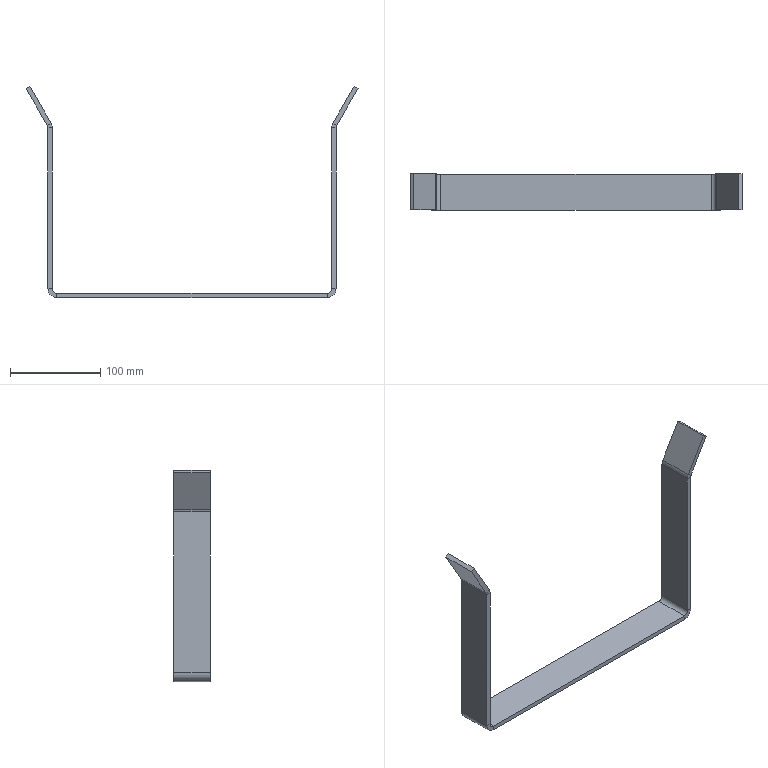Part | SolidWorks | features EdgeFlange 2, FlatPattern 1, SMBaseFlange 1, SheetMetal 1 | 1 solid | 38 faces | box 368.66 x 40 x 234.641 mm | volume 156675 mm3 | plane 30 | cylinder 8 | commonest cylinder face diameters 10 x4 20 x4
STEP:
#1=CARTESIAN_POINT('',(160.,-20.,5.));
#2=VERTEX_POINT('',#1);
#3=CARTESIAN_POINT('',(160.,-20.,183.66));
#4=VERTEX_POINT('',#3);
#5=CARTESIAN_POINT('',(160.,-20.,0.));
#6=DIRECTION('',(0.,0.,1.));
#7=VECTOR('',#6,1000.);
#8=LINE('',#5,#7);
#9=EDGE_CURVE('',#2,#4,#8,.T.);
#10=ORIENTED_EDGE('',*,*,#9,.T.);
#11=CARTESIAN_POINT('',(155.,-20.,183.66));
#12=VERTEX_POINT('',#11);
#13=CARTESIAN_POINT('',(160.,-20.,183.66));
#14=DIRECTION('',(-1.,0.,0.));
#15=VECTOR('',#14,1000.);
#16=LINE('',#13,#15);
#17=EDGE_CURVE('',#4,#12,#16,.T.);
#18=ORIENTED_EDGE('',*,*,#17,.T.);
#19=CARTESIAN_POINT('',(155.,-20.,5.));
#20=VERTEX_POINT('',#19);
#21=CARTESIAN_POINT('',(155.,-20.,0.));
#22=DIRECTION('',(0.,0.,1.));
#23=VECTOR('',#22,1000.);
#24=LINE('',#21,#23);
#25=EDGE_CURVE('',#20,#12,#24,.T.);
#26=ORIENTED_EDGE('',*,*,#25,.F.);
#27=CARTESIAN_POINT('',(160.,-20.,5.));
#28=DIRECTION('',(1.,0.,0.));
#29=VECTOR('',#28,1000.);
#30=LINE('',#27,#29);
#31=EDGE_CURVE('',#20,#2,#30,.T.);
#32=ORIENTED_EDGE('',*,*,#31,.T.);
#33=EDGE_LOOP('',(#10,#18,#26,#32));
#34=FACE_OUTER_BOUND('',#33,.T.);
#35=CARTESIAN_POINT('',(160.,-20.,0.));
#36=DIRECTION('',(0.,-1.,0.));
#37=DIRECTION('',(0.,0.,-1.));
#38=AXIS2_PLACEMENT_3D('',#35,#36,#37);
#39=PLANE('',#38);
#40=ADVANCED_FACE('',(#34),#39,.T.);
#41=CARTESIAN_POINT('',(160.,20.,183.66));
#42=VERTEX_POINT('',#41);
#43=CARTESIAN_POINT('',(160.,-20.,183.66));
#44=DIRECTION('',(0.,1.,0.));
#45=VECTOR('',#44,1000.);
#46=LINE('',#43,#45);
#47=EDGE_CURVE('',#4,#42,#46,.T.);
#48=ORIENTED_EDGE('',*,*,#47,.F.);
#49=ORIENTED_EDGE('',*,*,#9,.F.);
#50=CARTESIAN_POINT('',(160.,20.,5.));
#51=VERTEX_POINT('',#50);
#52=CARTESIAN_POINT('',(160.,-20.,5.));
#53=DIRECTION('',(0.,-1.,0.));
#54=VECTOR('',#53,1000.);
#55=LINE('',#52,#54);
#56=EDGE_CURVE('',#51,#2,#55,.T.);
#57=ORIENTED_EDGE('',*,*,#56,.F.);
#58=CARTESIAN_POINT('',(160.,20.,195.));
#59=DIRECTION('',(0.,0.,-1.));
#60=VECTOR('',#59,1000.);
#61=LINE('',#58,#60);
#62=EDGE_CURVE('',#42,#51,#61,.T.);
#63=ORIENTED_EDGE('',*,*,#62,.F.);
#64=EDGE_LOOP('',(#48,#49,#57,#63));
#65=FACE_OUTER_BOUND('',#64,.T.);
#66=CARTESIAN_POINT('',(160.,0.,0.));
#67=DIRECTION('',(-1.,0.,0.));
#68=DIRECTION('',(0.,0.,1.));
#69=AXIS2_PLACEMENT_3D('',#66,#67,#68);
#70=PLANE('',#69);
#71=ADVANCED_FACE('',(#65),#70,.F.);
#72=ORIENTED_EDGE('',*,*,#25,.T.);
#73=CARTESIAN_POINT('',(155.,20.,183.66));
#74=VERTEX_POINT('',#73);
#75=CARTESIAN_POINT('',(155.,-20.,183.66));
#76=DIRECTION('',(0.,1.,0.));
#77=VECTOR('',#76,1000.);
#78=LINE('',#75,#77);
#79=EDGE_CURVE('',#12,#74,#78,.T.);
#80=ORIENTED_EDGE('',*,*,#79,.T.);
#81=CARTESIAN_POINT('',(155.,20.,5.));
#82=VERTEX_POINT('',#81);
#83=CARTESIAN_POINT('',(155.,20.,0.));
#84=DIRECTION('',(0.,0.,-1.));
#85=VECTOR('',#84,1000.);
#86=LINE('',#83,#85);
#87=EDGE_CURVE('',#74,#82,#86,.T.);
#88=ORIENTED_EDGE('',*,*,#87,.T.);
#89=CARTESIAN_POINT('',(155.,-20.,5.));
#90=DIRECTION('',(0.,1.,0.));
#91=VECTOR('',#90,1000.);
#92=LINE('',#89,#91);
#93=EDGE_CURVE('',#20,#82,#92,.T.);
#94=ORIENTED_EDGE('',*,*,#93,.F.);
#95=EDGE_LOOP('',(#72,#80,#88,#94));
#96=FACE_OUTER_BOUND('',#95,.T.);
#97=CARTESIAN_POINT('',(155.,0.,0.));
#98=DIRECTION('',(-1.,0.,0.));
#99=DIRECTION('',(0.,0.,1.));
#100=AXIS2_PLACEMENT_3D('',#97,#98,#99);
#101=PLANE('',#100);
#102=ADVANCED_FACE('',(#96),#101,.T.);
#103=CARTESIAN_POINT('',(-160.,20.,5.));
#104=VERTEX_POINT('',#103);
#105=CARTESIAN_POINT('',(-160.,20.,183.66));
#106=VERTEX_POINT('',#105);
#107=CARTESIAN_POINT('',(-160.,20.,195.));
#108=DIRECTION('',(0.,0.,1.));
#109=VECTOR('',#108,1000.);
#110=LINE('',#107,#109);
#111=EDGE_CURVE('',#104,#106,#110,.T.);
#112=ORIENTED_EDGE('',*,*,#111,.T.);
#113=CARTESIAN_POINT('',(-155.,20.,183.66));
#114=VERTEX_POINT('',#113);
#115=CARTESIAN_POINT('',(-160.,20.,183.66));
#116=DIRECTION('',(1.,0.,0.));
#117=VECTOR('',#116,1000.);
#118=LINE('',#115,#117);
#119=EDGE_CURVE('',#106,#114,#118,.T.);
#120=ORIENTED_EDGE('',*,*,#119,.T.);
#121=CARTESIAN_POINT('',(-155.,20.,5.));
#122=VERTEX_POINT('',#121);
#123=CARTESIAN_POINT('',(-155.,20.,0.));
#124=DIRECTION('',(0.,0.,1.));
#125=VECTOR('',#124,1000.);
#126=LINE('',#123,#125);
#127=EDGE_CURVE('',#122,#114,#126,.T.);
#128=ORIENTED_EDGE('',*,*,#127,.F.);
#129=CARTESIAN_POINT('',(-160.,20.,5.));
#130=DIRECTION('',(-1.,0.,0.));
#131=VECTOR('',#130,1000.);
#132=LINE('',#129,#131);
#133=EDGE_CURVE('',#122,#104,#132,.T.);
#134=ORIENTED_EDGE('',*,*,#133,.T.);
#135=EDGE_LOOP('',(#112,#120,#128,#134));
#136=FACE_OUTER_BOUND('',#135,.T.);
#137=CARTESIAN_POINT('',(-160.,20.,195.));
#138=DIRECTION('',(0.,1.,0.));
#139=DIRECTION('',(0.,0.,1.));
#140=AXIS2_PLACEMENT_3D('',#137,#138,#139);
#141=PLANE('',#140);
#142=ADVANCED_FACE('',(#136),#141,.T.);
#143=CARTESIAN_POINT('',(-160.,-20.,183.66));
#144=VERTEX_POINT('',#143);
#145=CARTESIAN_POINT('',(-160.,-20.,5.));
#146=VERTEX_POINT('',#145);
#147=CARTESIAN_POINT('',(-160.,-20.,0.));
#148=DIRECTION('',(0.,0.,-1.));
#149=VECTOR('',#148,1000.);
#150=LINE('',#147,#149);
#151=EDGE_CURVE('',#144,#146,#150,.T.);
#152=ORIENTED_EDGE('',*,*,#151,.F.);
#153=CARTESIAN_POINT('',(-160.,20.,183.66));
#154=DIRECTION('',(0.,-1.,0.));
#155=VECTOR('',#154,1000.);
#156=LINE('',#153,#155);
#157=EDGE_CURVE('',#106,#144,#156,.T.);
#158=ORIENTED_EDGE('',*,*,#157,.F.);
#159=ORIENTED_EDGE('',*,*,#111,.F.);
#160=CARTESIAN_POINT('',(-160.,0.,5.));
#161=DIRECTION('',(0.,-1.,0.));
#162=VECTOR('',#161,1000.);
#163=LINE('',#160,#162);
#164=EDGE_CURVE('',#104,#146,#163,.T.);
#165=ORIENTED_EDGE('',*,*,#164,.T.);
#166=EDGE_LOOP('',(#152,#158,#159,#165));
#167=FACE_OUTER_BOUND('',#166,.T.);
#168=CARTESIAN_POINT('',(-160.,0.,0.));
#169=DIRECTION('',(-1.,0.,0.));
#170=DIRECTION('',(0.,0.,1.));
#171=AXIS2_PLACEMENT_3D('',#168,#169,#170);
#172=PLANE('',#171);
#173=ADVANCED_FACE('',(#167),#172,.T.);
#174=CARTESIAN_POINT('',(-155.,-20.,183.66));
#175=VERTEX_POINT('',#174);
#176=CARTESIAN_POINT('',(-155.,20.,183.66));
#177=DIRECTION('',(0.,-1.,0.));
#178=VECTOR('',#177,1000.);
#179=LINE('',#176,#178);
#180=EDGE_CURVE('',#114,#175,#179,.T.);
#181=ORIENTED_EDGE('',*,*,#180,.T.);
#182=CARTESIAN_POINT('',(-155.,-20.,5.));
#183=VERTEX_POINT('',#182);
#184=CARTESIAN_POINT('',(-155.,-20.,0.));
#185=DIRECTION('',(0.,0.,-1.));
#186=VECTOR('',#185,1000.);
#187=LINE('',#184,#186);
#188=EDGE_CURVE('',#175,#183,#187,.T.);
#189=ORIENTED_EDGE('',*,*,#188,.T.);
#190=CARTESIAN_POINT('',(-155.,20.,5.));
#191=DIRECTION('',(0.,-1.,0.));
#192=VECTOR('',#191,1000.);
#193=LINE('',#190,#192);
#194=EDGE_CURVE('',#122,#183,#193,.T.);
#195=ORIENTED_EDGE('',*,*,#194,.F.);
#196=ORIENTED_EDGE('',*,*,#127,.T.);
#197=EDGE_LOOP('',(#181,#189,#195,#196));
#198=FACE_OUTER_BOUND('',#197,.T.);
#199=CARTESIAN_POINT('',(-155.,0.,0.));
#200=DIRECTION('',(-1.,0.,0.));
#201=DIRECTION('',(0.,0.,1.));
#202=AXIS2_PLACEMENT_3D('',#199,#200,#201);
#203=PLANE('',#202);
#204=ADVANCED_FACE('',(#198),#203,.F.);
#205=CARTESIAN_POINT('',(150.,20.,-5.));
#206=VERTEX_POINT('',#205);
#207=CARTESIAN_POINT('',(150.,-20.,-5.));
#208=VERTEX_POINT('',#207);
#209=CARTESIAN_POINT('',(150.,20.,-5.));
#210=DIRECTION('',(0.,-1.,0.));
#211=VECTOR('',#210,1000.);
#212=LINE('',#209,#211);
#213=EDGE_CURVE('',#206,#208,#212,.T.);
#214=ORIENTED_EDGE('',*,*,#213,.T.);
#215=CARTESIAN_POINT('',(-150.,-20.,-5.));
#216=VERTEX_POINT('',#215);
#217=CARTESIAN_POINT('',(-160.,-20.,-5.));
#218=DIRECTION('',(1.,0.,0.));
#219=VECTOR('',#218,1000.);
#220=LINE('',#217,#219);
#221=EDGE_CURVE('',#216,#208,#220,.T.);
#222=ORIENTED_EDGE('',*,*,#221,.F.);
#223=CARTESIAN_POINT('',(-150.,20.,-5.));
#224=VERTEX_POINT('',#223);
#225=CARTESIAN_POINT('',(-150.,-20.,-5.));
#226=DIRECTION('',(0.,1.,0.));
#227=VECTOR('',#226,1000.);
#228=LINE('',#225,#227);
#229=EDGE_CURVE('',#216,#224,#228,.T.);
#230=ORIENTED_EDGE('',*,*,#229,.T.);
#231=CARTESIAN_POINT('',(-160.,20.,-5.));
#232=DIRECTION('',(-1.,0.,0.));
#233=VECTOR('',#232,1000.);
#234=LINE('',#231,#233);
#235=EDGE_CURVE('',#206,#224,#234,.T.);
#236=ORIENTED_EDGE('',*,*,#235,.F.);
#237=EDGE_LOOP('',(#214,#222,#230,#236));
#238=FACE_OUTER_BOUND('',#237,.T.);
#239=CARTESIAN_POINT('',(0.,0.,-5.));
#240=DIRECTION('',(0.,0.,1.));
#241=DIRECTION('',(1.,0.,0.));
#242=AXIS2_PLACEMENT_3D('',#239,#240,#241);
#243=PLANE('',#242);
#244=ADVANCED_FACE('',(#238),#243,.F.);
#245=CARTESIAN_POINT('',(-150.,-20.,0.));
#246=VERTEX_POINT('',#245);
#247=CARTESIAN_POINT('',(150.,-20.,0.));
#248=VERTEX_POINT('',#247);
#249=CARTESIAN_POINT('',(-160.,-20.,0.));
#250=DIRECTION('',(1.,0.,0.));
#251=VECTOR('',#250,1000.);
#252=LINE('',#249,#251);
#253=EDGE_CURVE('',#246,#248,#252,.T.);
#254=ORIENTED_EDGE('',*,*,#253,.T.);
#255=CARTESIAN_POINT('',(150.,20.,0.));
#256=VERTEX_POINT('',#255);
#257=CARTESIAN_POINT('',(150.,20.,0.));
#258=DIRECTION('',(0.,-1.,0.));
#259=VECTOR('',#258,1000.);
#260=LINE('',#257,#259);
#261=EDGE_CURVE('',#256,#248,#260,.T.);
#262=ORIENTED_EDGE('',*,*,#261,.F.);
#263=CARTESIAN_POINT('',(-150.,20.,0.));
#264=VERTEX_POINT('',#263);
#265=CARTESIAN_POINT('',(-160.,20.,0.));
#266=DIRECTION('',(-1.,0.,0.));
#267=VECTOR('',#266,1000.);
#268=LINE('',#265,#267);
#269=EDGE_CURVE('',#256,#264,#268,.T.);
#270=ORIENTED_EDGE('',*,*,#269,.T.);
#271=CARTESIAN_POINT('',(-150.,-20.,0.));
#272=DIRECTION('',(0.,1.,0.));
#273=VECTOR('',#272,1000.);
#274=LINE('',#271,#273);
#275=EDGE_CURVE('',#246,#264,#274,.T.);
#276=ORIENTED_EDGE('',*,*,#275,.F.);
#277=EDGE_LOOP('',(#254,#262,#270,#276));
#278=FACE_OUTER_BOUND('',#277,.T.);
#279=CARTESIAN_POINT('',(0.,0.,0.));
#280=DIRECTION('',(0.,0.,1.));
#281=DIRECTION('',(1.,0.,0.));
#282=AXIS2_PLACEMENT_3D('',#279,#280,#281);
#283=PLANE('',#282);
#284=ADVANCED_FACE('',(#278),#283,.T.);
#285=ORIENTED_EDGE('',*,*,#269,.F.);
#286=CARTESIAN_POINT('',(150.,20.,0.));
#287=DIRECTION('',(0.,0.,-1.));
#288=VECTOR('',#287,1000.);
#289=LINE('',#286,#288);
#290=EDGE_CURVE('',#256,#206,#289,.T.);
#291=ORIENTED_EDGE('',*,*,#290,.T.);
#292=ORIENTED_EDGE('',*,*,#235,.T.);
#293=CARTESIAN_POINT('',(-150.,20.,0.));
#294=DIRECTION('',(0.,0.,-1.));
#295=VECTOR('',#294,1000.);
#296=LINE('',#293,#295);
#297=EDGE_CURVE('',#264,#224,#296,.T.);
#298=ORIENTED_EDGE('',*,*,#297,.F.);
#299=EDGE_LOOP('',(#285,#291,#292,#298));
#300=FACE_OUTER_BOUND('',#299,.T.);
#301=CARTESIAN_POINT('',(-160.,20.,-5.));
#302=DIRECTION('',(0.,1.,0.));
#303=DIRECTION('',(0.,0.,1.));
#304=AXIS2_PLACEMENT_3D('',#301,#302,#303);
#305=PLANE('',#304);
#306=ADVANCED_FACE('',(#300),#305,.T.);
#307=CARTESIAN_POINT('',(150.,-20.,0.));
#308=DIRECTION('',(0.,0.,-1.));
#309=VECTOR('',#308,1000.);
#310=LINE('',#307,#309);
#311=EDGE_CURVE('',#248,#208,#310,.T.);
#312=ORIENTED_EDGE('',*,*,#311,.F.);
#313=ORIENTED_EDGE('',*,*,#253,.F.);
#314=CARTESIAN_POINT('',(-150.,-20.,0.));
#315=DIRECTION('',(0.,0.,-1.));
#316=VECTOR('',#315,1000.);
#317=LINE('',#314,#316);
#318=EDGE_CURVE('',#246,#216,#317,.T.);
#319=ORIENTED_EDGE('',*,*,#318,.T.);
#320=ORIENTED_EDGE('',*,*,#221,.T.);
#321=EDGE_LOOP('',(#312,#313,#319,#320));
#322=FACE_OUTER_BOUND('',#321,.T.);
#323=CARTESIAN_POINT('',(-160.,-20.,-5.));
#324=DIRECTION('',(0.,-1.,0.));
#325=DIRECTION('',(0.,0.,-1.));
#326=AXIS2_PLACEMENT_3D('',#323,#324,#325);
#327=PLANE('',#326);
#328=ADVANCED_FACE('',(#322),#327,.T.);
#329=ORIENTED_EDGE('',*,*,#133,.F.);
#330=CARTESIAN_POINT('',(-150.,20.,5.));
#331=DIRECTION('',(0.,1.,0.));
#332=DIRECTION('',(0.,0.,-1.));
#333=AXIS2_PLACEMENT_3D('',#330,#331,#332);
#334=CIRCLE('',#333,5.);
#335=EDGE_CURVE('',#264,#122,#334,.T.);
#336=ORIENTED_EDGE('',*,*,#335,.F.);
#337=ORIENTED_EDGE('',*,*,#297,.T.);
#338=CARTESIAN_POINT('',(-150.,20.,5.));
#339=DIRECTION('',(0.,1.,0.));
#340=DIRECTION('',(0.,0.,-1.));
#341=AXIS2_PLACEMENT_3D('',#338,#339,#340);
#342=CIRCLE('',#341,10.);
#343=EDGE_CURVE('',#224,#104,#342,.T.);
#344=ORIENTED_EDGE('',*,*,#343,.T.);
#345=EDGE_LOOP('',(#329,#336,#337,#344));
#346=FACE_OUTER_BOUND('',#345,.T.);
#347=CARTESIAN_POINT('',(-150.,20.,5.));
#348=DIRECTION('',(0.,1.,0.));
#349=DIRECTION('',(0.,0.,1.));
#350=AXIS2_PLACEMENT_3D('',#347,#348,#349);
#351=PLANE('',#350);
#352=ADVANCED_FACE('',(#346),#351,.T.);
#353=CARTESIAN_POINT('',(-150.,-20.,5.));
#354=DIRECTION('',(0.,-1.,0.));
#355=DIRECTION('',(0.,0.,-1.));
#356=AXIS2_PLACEMENT_3D('',#353,#354,#355);
#357=CIRCLE('',#356,5.);
#358=EDGE_CURVE('',#183,#246,#357,.T.);
#359=ORIENTED_EDGE('',*,*,#358,.F.);
#360=CARTESIAN_POINT('',(-155.,-20.,5.));
#361=DIRECTION('',(-1.,0.,0.));
#362=VECTOR('',#361,1000.);
#363=LINE('',#360,#362);
#364=EDGE_CURVE('',#183,#146,#363,.T.);
#365=ORIENTED_EDGE('',*,*,#364,.T.);
#366=CARTESIAN_POINT('',(-150.,-20.,5.));
#367=DIRECTION('',(0.,-1.,0.));
#368=DIRECTION('',(0.,0.,-1.));
#369=AXIS2_PLACEMENT_3D('',#366,#367,#368);
#370=CIRCLE('',#369,10.);
#371=EDGE_CURVE('',#146,#216,#370,.T.);
#372=ORIENTED_EDGE('',*,*,#371,.T.);
#373=ORIENTED_EDGE('',*,*,#318,.F.);
#374=EDGE_LOOP('',(#359,#365,#372,#373));
#375=FACE_OUTER_BOUND('',#374,.T.);
#376=CARTESIAN_POINT('',(-150.,-20.,5.));
#377=DIRECTION('',(0.,1.,0.));
#378=DIRECTION('',(0.,0.,1.));
#379=AXIS2_PLACEMENT_3D('',#376,#377,#378);
#380=PLANE('',#379);
#381=ADVANCED_FACE('',(#375),#380,.F.);
#382=ORIENTED_EDGE('',*,*,#229,.F.);
#383=ORIENTED_EDGE('',*,*,#371,.F.);
#384=ORIENTED_EDGE('',*,*,#164,.F.);
#385=ORIENTED_EDGE('',*,*,#343,.F.);
#386=EDGE_LOOP('',(#382,#383,#384,#385));
#387=FACE_OUTER_BOUND('',#386,.T.);
#388=CARTESIAN_POINT('',(-150.,-20.,5.));
#389=DIRECTION('',(0.,-1.,0.));
#390=DIRECTION('',(-1.,0.,0.));
#391=AXIS2_PLACEMENT_3D('',#388,#389,#390);
#392=CYLINDRICAL_SURFACE('',#391,10.);
#393=ADVANCED_FACE('',(#387),#392,.T.);
#394=ORIENTED_EDGE('',*,*,#275,.T.);
#395=ORIENTED_EDGE('',*,*,#335,.T.);
#396=ORIENTED_EDGE('',*,*,#194,.T.);
#397=ORIENTED_EDGE('',*,*,#358,.T.);
#398=EDGE_LOOP('',(#394,#395,#396,#397));
#399=FACE_OUTER_BOUND('',#398,.T.);
#400=CARTESIAN_POINT('',(-150.,-20.,5.));
#401=DIRECTION('',(0.,-1.,0.));
#402=DIRECTION('',(-1.,0.,0.));
#403=AXIS2_PLACEMENT_3D('',#400,#401,#402);
#404=CYLINDRICAL_SURFACE('',#403,5.);
#405=ADVANCED_FACE('',(#399),#404,.F.);
#406=CARTESIAN_POINT('',(-160.,-20.,183.66));
#407=DIRECTION('',(1.,0.,0.));
#408=VECTOR('',#407,1000.);
#409=LINE('',#406,#408);
#410=EDGE_CURVE('',#144,#175,#409,.T.);
#411=ORIENTED_EDGE('',*,*,#410,.F.);
#412=ORIENTED_EDGE('',*,*,#151,.T.);
#413=ORIENTED_EDGE('',*,*,#364,.F.);
#414=ORIENTED_EDGE('',*,*,#188,.F.);
#415=EDGE_LOOP('',(#411,#412,#413,#414));
#416=FACE_OUTER_BOUND('',#415,.T.);
#417=CARTESIAN_POINT('',(-160.,-20.,0.));
#418=DIRECTION('',(0.,-1.,0.));
#419=DIRECTION('',(0.,0.,-1.));
#420=AXIS2_PLACEMENT_3D('',#417,#418,#419);
#421=PLANE('',#420);
#422=ADVANCED_FACE('',(#416),#421,.T.);
#423=ORIENTED_EDGE('',*,*,#31,.F.);
#424=CARTESIAN_POINT('',(150.,-20.,5.));
#425=DIRECTION('',(0.,-1.,0.));
#426=DIRECTION('',(0.,0.,1.));
#427=AXIS2_PLACEMENT_3D('',#424,#425,#426);
#428=CIRCLE('',#427,5.);
#429=EDGE_CURVE('',#248,#20,#428,.T.);
#430=ORIENTED_EDGE('',*,*,#429,.F.);
#431=ORIENTED_EDGE('',*,*,#311,.T.);
#432=CARTESIAN_POINT('',(150.,-20.,5.));
#433=DIRECTION('',(0.,-1.,0.));
#434=DIRECTION('',(0.,0.,1.));
#435=AXIS2_PLACEMENT_3D('',#432,#433,#434);
#436=CIRCLE('',#435,10.);
#437=EDGE_CURVE('',#208,#2,#436,.T.);
#438=ORIENTED_EDGE('',*,*,#437,.T.);
#439=EDGE_LOOP('',(#423,#430,#431,#438));
#440=FACE_OUTER_BOUND('',#439,.T.);
#441=CARTESIAN_POINT('',(150.,-20.,5.));
#442=DIRECTION('',(0.,-1.,0.));
#443=DIRECTION('',(0.,0.,-1.));
#444=AXIS2_PLACEMENT_3D('',#441,#442,#443);
#445=PLANE('',#444);
#446=ADVANCED_FACE('',(#440),#445,.T.);
#447=CARTESIAN_POINT('',(150.,20.,5.));
#448=DIRECTION('',(0.,1.,0.));
#449=DIRECTION('',(0.,0.,1.));
#450=AXIS2_PLACEMENT_3D('',#447,#448,#449);
#451=CIRCLE('',#450,5.);
#452=EDGE_CURVE('',#82,#256,#451,.T.);
#453=ORIENTED_EDGE('',*,*,#452,.F.);
#454=CARTESIAN_POINT('',(155.,20.,5.));
#455=DIRECTION('',(1.,0.,0.));
#456=VECTOR('',#455,1000.);
#457=LINE('',#454,#456);
#458=EDGE_CURVE('',#82,#51,#457,.T.);
#459=ORIENTED_EDGE('',*,*,#458,.T.);
#460=CARTESIAN_POINT('',(150.,20.,5.));
#461=DIRECTION('',(0.,1.,0.));
#462=DIRECTION('',(0.,0.,1.));
#463=AXIS2_PLACEMENT_3D('',#460,#461,#462);
#464=CIRCLE('',#463,10.);
#465=EDGE_CURVE('',#51,#206,#464,.T.);
#466=ORIENTED_EDGE('',*,*,#465,.T.);
#467=ORIENTED_EDGE('',*,*,#290,.F.);
#468=EDGE_LOOP('',(#453,#459,#466,#467));
#469=FACE_OUTER_BOUND('',#468,.T.);
#470=CARTESIAN_POINT('',(150.,20.,5.));
#471=DIRECTION('',(0.,-1.,0.));
#472=DIRECTION('',(0.,0.,-1.));
#473=AXIS2_PLACEMENT_3D('',#470,#471,#472);
#474=PLANE('',#473);
#475=ADVANCED_FACE('',(#469),#474,.F.);
#476=ORIENTED_EDGE('',*,*,#213,.F.);
#477=ORIENTED_EDGE('',*,*,#465,.F.);
#478=ORIENTED_EDGE('',*,*,#56,.T.);
#479=ORIENTED_EDGE('',*,*,#437,.F.);
#480=EDGE_LOOP('',(#476,#477,#478,#479));
#481=FACE_OUTER_BOUND('',#480,.T.);
#482=CARTESIAN_POINT('',(150.,20.,5.));
#483=DIRECTION('',(0.,1.,0.));
#484=DIRECTION('',(1.,0.,0.));
#485=AXIS2_PLACEMENT_3D('',#482,#483,#484);
#486=CYLINDRICAL_SURFACE('',#485,10.);
#487=ADVANCED_FACE('',(#481),#486,.T.);
#488=ORIENTED_EDGE('',*,*,#261,.T.);
#489=ORIENTED_EDGE('',*,*,#429,.T.);
#490=ORIENTED_EDGE('',*,*,#93,.T.);
#491=ORIENTED_EDGE('',*,*,#452,.T.);
#492=EDGE_LOOP('',(#488,#489,#490,#491));
#493=FACE_OUTER_BOUND('',#492,.T.);
#494=CARTESIAN_POINT('',(150.,20.,5.));
#495=DIRECTION('',(0.,1.,0.));
#496=DIRECTION('',(1.,0.,0.));
#497=AXIS2_PLACEMENT_3D('',#494,#495,#496);
#498=CYLINDRICAL_SURFACE('',#497,5.);
#499=ADVANCED_FACE('',(#493),#498,.F.);
#500=CARTESIAN_POINT('',(160.,20.,183.66));
#501=DIRECTION('',(-1.,0.,0.));
#502=VECTOR('',#501,1000.);
#503=LINE('',#500,#502);
#504=EDGE_CURVE('',#42,#74,#503,.T.);
#505=ORIENTED_EDGE('',*,*,#504,.F.);
#506=ORIENTED_EDGE('',*,*,#62,.T.);
#507=ORIENTED_EDGE('',*,*,#458,.F.);
#508=ORIENTED_EDGE('',*,*,#87,.F.);
#509=EDGE_LOOP('',(#505,#506,#507,#508));
#510=FACE_OUTER_BOUND('',#509,.T.);
#511=CARTESIAN_POINT('',(160.,20.,195.));
#512=DIRECTION('',(0.,1.,0.));
#513=DIRECTION('',(0.,0.,1.));
#514=AXIS2_PLACEMENT_3D('',#511,#512,#513);
#515=PLANE('',#514);
#516=ADVANCED_FACE('',(#510),#515,.T.);
#517=CARTESIAN_POINT('',(-160.67,-20.,186.16));
#518=VERTEX_POINT('',#517);
#519=CARTESIAN_POINT('',(-156.34,-20.,188.66));
#520=VERTEX_POINT('',#519);
#521=CARTESIAN_POINT('',(-156.34,-20.,188.66));
#522=DIRECTION('',(0.866,0.,0.5));
#523=VECTOR('',#522,1000.);
#524=LINE('',#521,#523);
#525=EDGE_CURVE('',#518,#520,#524,.T.);
#526=ORIENTED_EDGE('',*,*,#525,.F.);
#527=CARTESIAN_POINT('',(-165.,-20.,183.66));
#528=DIRECTION('',(0.,-1.,0.));
#529=DIRECTION('',(0.,0.,1.));
#530=AXIS2_PLACEMENT_3D('',#527,#528,#529);
#531=CIRCLE('',#530,5.);
#532=EDGE_CURVE('',#144,#518,#531,.T.);
#533=ORIENTED_EDGE('',*,*,#532,.F.);
#534=ORIENTED_EDGE('',*,*,#410,.T.);
#535=CARTESIAN_POINT('',(-165.,-20.,183.66));
#536=DIRECTION('',(0.,-1.,0.));
#537=DIRECTION('',(0.,0.,1.));
#538=AXIS2_PLACEMENT_3D('',#535,#536,#537);
#539=CIRCLE('',#538,10.);
#540=EDGE_CURVE('',#175,#520,#539,.T.);
#541=ORIENTED_EDGE('',*,*,#540,.T.);
#542=EDGE_LOOP('',(#526,#533,#534,#541));
#543=FACE_OUTER_BOUND('',#542,.T.);
#544=CARTESIAN_POINT('',(-165.,-20.,183.66));
#545=DIRECTION('',(0.,-1.,0.));
#546=DIRECTION('',(0.,0.,-1.));
#547=AXIS2_PLACEMENT_3D('',#544,#545,#546);
#548=PLANE('',#547);
#549=ADVANCED_FACE('',(#543),#548,.T.);
#550=CARTESIAN_POINT('',(-160.67,20.,186.16));
#551=VERTEX_POINT('',#550);
#552=CARTESIAN_POINT('',(-165.,20.,183.66));
#553=DIRECTION('',(0.,1.,0.));
#554=DIRECTION('',(0.,0.,1.));
#555=AXIS2_PLACEMENT_3D('',#552,#553,#554);
#556=CIRCLE('',#555,5.);
#557=EDGE_CURVE('',#551,#106,#556,.T.);
#558=ORIENTED_EDGE('',*,*,#557,.F.);
#559=CARTESIAN_POINT('',(-156.34,20.,188.66));
#560=VERTEX_POINT('',#559);
#561=CARTESIAN_POINT('',(-160.67,20.,186.16));
#562=DIRECTION('',(0.866,0.,0.5));
#563=VECTOR('',#562,1000.);
#564=LINE('',#561,#563);
#565=EDGE_CURVE('',#551,#560,#564,.T.);
#566=ORIENTED_EDGE('',*,*,#565,.T.);
#567=CARTESIAN_POINT('',(-165.,20.,183.66));
#568=DIRECTION('',(0.,1.,0.));
#569=DIRECTION('',(0.,0.,1.));
#570=AXIS2_PLACEMENT_3D('',#567,#568,#569);
#571=CIRCLE('',#570,10.);
#572=EDGE_CURVE('',#560,#114,#571,.T.);
#573=ORIENTED_EDGE('',*,*,#572,.T.);
#574=ORIENTED_EDGE('',*,*,#119,.F.);
#575=EDGE_LOOP('',(#558,#566,#573,#574));
#576=FACE_OUTER_BOUND('',#575,.T.);
#577=CARTESIAN_POINT('',(-165.,20.,183.66));
#578=DIRECTION('',(0.,-1.,0.));
#579=DIRECTION('',(0.,0.,-1.));
#580=AXIS2_PLACEMENT_3D('',#577,#578,#579);
#581=PLANE('',#580);
#582=ADVANCED_FACE('',(#576),#581,.F.);
#583=ORIENTED_EDGE('',*,*,#180,.F.);
#584=ORIENTED_EDGE('',*,*,#572,.F.);
#585=CARTESIAN_POINT('',(-156.34,0.,188.66));
#586=DIRECTION('',(0.,1.,0.));
#587=VECTOR('',#586,1000.);
#588=LINE('',#585,#587);
#589=EDGE_CURVE('',#520,#560,#588,.T.);
#590=ORIENTED_EDGE('',*,*,#589,.F.);
#591=ORIENTED_EDGE('',*,*,#540,.F.);
#592=EDGE_LOOP('',(#583,#584,#590,#591));
#593=FACE_OUTER_BOUND('',#592,.T.);
#594=CARTESIAN_POINT('',(-165.,20.,183.66));
#595=DIRECTION('',(0.,1.,0.));
#596=DIRECTION('',(0.866,0.,0.5));
#597=AXIS2_PLACEMENT_3D('',#594,#595,#596);
#598=CYLINDRICAL_SURFACE('',#597,10.);
#599=ADVANCED_FACE('',(#593),#598,.T.);
#600=ORIENTED_EDGE('',*,*,#157,.T.);
#601=ORIENTED_EDGE('',*,*,#532,.T.);
#602=CARTESIAN_POINT('',(-160.67,-20.,186.16));
#603=DIRECTION('',(0.,1.,0.));
#604=VECTOR('',#603,1000.);
#605=LINE('',#602,#604);
#606=EDGE_CURVE('',#518,#551,#605,.T.);
#607=ORIENTED_EDGE('',*,*,#606,.T.);
#608=ORIENTED_EDGE('',*,*,#557,.T.);
#609=EDGE_LOOP('',(#600,#601,#607,#608));
#610=FACE_OUTER_BOUND('',#609,.T.);
#611=CARTESIAN_POINT('',(-165.,20.,183.66));
#612=DIRECTION('',(0.,1.,0.));
#613=DIRECTION('',(0.866,0.,0.5));
#614=AXIS2_PLACEMENT_3D('',#611,#612,#613);
#615=CYLINDRICAL_SURFACE('',#614,5.);
#616=ADVANCED_FACE('',(#610),#615,.F.);
#617=CARTESIAN_POINT('',(-180.,20.,229.641));
#618=VERTEX_POINT('',#617);
#619=CARTESIAN_POINT('',(-155.67,20.,187.5));
#620=DIRECTION('',(0.5,0.,-0.866));
#621=VECTOR('',#620,1000.);
#622=LINE('',#619,#621);
#623=EDGE_CURVE('',#618,#560,#622,.T.);
#624=ORIENTED_EDGE('',*,*,#623,.T.);
#625=ORIENTED_EDGE('',*,*,#565,.F.);
#626=CARTESIAN_POINT('',(-184.33,20.,227.141));
#627=VERTEX_POINT('',#626);
#628=CARTESIAN_POINT('',(-35.563,20.,-30.532));
#629=DIRECTION('',(0.5,0.,-0.866));
#630=VECTOR('',#629,1000.);
#631=LINE('',#628,#630);
#632=EDGE_CURVE('',#627,#551,#631,.T.);
#633=ORIENTED_EDGE('',*,*,#632,.F.);
#634=CARTESIAN_POINT('',(-180.,20.,229.641));
#635=DIRECTION('',(-0.866,0.,-0.5));
#636=VECTOR('',#635,1000.);
#637=LINE('',#634,#636);
#638=EDGE_CURVE('',#618,#627,#637,.T.);
#639=ORIENTED_EDGE('',*,*,#638,.F.);
#640=EDGE_LOOP('',(#624,#625,#633,#639));
#641=FACE_OUTER_BOUND('',#640,.T.);
#642=CARTESIAN_POINT('',(-155.67,20.,187.5));
#643=DIRECTION('',(0.,1.,0.));
#644=DIRECTION('',(0.,0.,1.));
#645=AXIS2_PLACEMENT_3D('',#642,#643,#644);
#646=PLANE('',#645);
#647=ADVANCED_FACE('',(#641),#646,.T.);
#648=CARTESIAN_POINT('',(-184.33,-20.,227.141));
#649=VERTEX_POINT('',#648);
#650=CARTESIAN_POINT('',(-35.563,-20.,-30.532));
#651=DIRECTION('',(-0.5,0.,0.866));
#652=VECTOR('',#651,1000.);
#653=LINE('',#650,#652);
#654=EDGE_CURVE('',#518,#649,#653,.T.);
#655=ORIENTED_EDGE('',*,*,#654,.F.);
#656=ORIENTED_EDGE('',*,*,#525,.T.);
#657=CARTESIAN_POINT('',(-180.,-20.,229.641));
#658=VERTEX_POINT('',#657);
#659=CARTESIAN_POINT('',(-180.,-20.,229.641));
#660=DIRECTION('',(-0.5,0.,0.866));
#661=VECTOR('',#660,1000.);
#662=LINE('',#659,#661);
#663=EDGE_CURVE('',#520,#658,#662,.T.);
#664=ORIENTED_EDGE('',*,*,#663,.T.);
#665=CARTESIAN_POINT('',(-180.,-20.,229.641));
#666=DIRECTION('',(-0.866,0.,-0.5));
#667=VECTOR('',#666,1000.);
#668=LINE('',#665,#667);
#669=EDGE_CURVE('',#658,#649,#668,.T.);
#670=ORIENTED_EDGE('',*,*,#669,.T.);
#671=EDGE_LOOP('',(#655,#656,#664,#670));
#672=FACE_OUTER_BOUND('',#671,.T.);
#673=CARTESIAN_POINT('',(-180.,-20.,229.641));
#674=DIRECTION('',(0.,-1.,0.));
#675=DIRECTION('',(0.,0.,-1.));
#676=AXIS2_PLACEMENT_3D('',#673,#674,#675);
#677=PLANE('',#676);
#678=ADVANCED_FACE('',(#672),#677,.T.);
#679=ORIENTED_EDGE('',*,*,#663,.F.);
#680=ORIENTED_EDGE('',*,*,#589,.T.);
#681=ORIENTED_EDGE('',*,*,#623,.F.);
#682=CARTESIAN_POINT('',(-180.,20.,229.641));
#683=DIRECTION('',(0.,1.,0.));
#684=VECTOR('',#683,1000.);
#685=LINE('',#682,#684);
#686=EDGE_CURVE('',#658,#618,#685,.T.);
#687=ORIENTED_EDGE('',*,*,#686,.F.);
#688=EDGE_LOOP('',(#679,#680,#681,#687));
#689=FACE_OUTER_BOUND('',#688,.T.);
#690=CARTESIAN_POINT('',(-31.232,0.,-28.032));
#691=DIRECTION('',(0.866,0.,0.5));
#692=DIRECTION('',(0.5,0.,-0.866));
#693=AXIS2_PLACEMENT_3D('',#690,#691,#692);
#694=PLANE('',#693);
#695=ADVANCED_FACE('',(#689),#694,.T.);
#696=ORIENTED_EDGE('',*,*,#606,.F.);
#697=ORIENTED_EDGE('',*,*,#654,.T.);
#698=CARTESIAN_POINT('',(-184.33,0.,227.141));
#699=DIRECTION('',(0.,1.,0.));
#700=VECTOR('',#699,1000.);
#701=LINE('',#698,#700);
#702=EDGE_CURVE('',#649,#627,#701,.T.);
#703=ORIENTED_EDGE('',*,*,#702,.T.);
#704=ORIENTED_EDGE('',*,*,#632,.T.);
#705=EDGE_LOOP('',(#696,#697,#703,#704));
#706=FACE_OUTER_BOUND('',#705,.T.);
#707=CARTESIAN_POINT('',(-35.563,0.,-30.532));
#708=DIRECTION('',(0.866,0.,0.5));
#709=DIRECTION('',(0.5,0.,-0.866));
#710=AXIS2_PLACEMENT_3D('',#707,#708,#709);
#711=PLANE('',#710);
#712=ADVANCED_FACE('',(#706),#711,.F.);
#713=ORIENTED_EDGE('',*,*,#702,.F.);
#714=ORIENTED_EDGE('',*,*,#669,.F.);
#715=ORIENTED_EDGE('',*,*,#686,.T.);
#716=ORIENTED_EDGE('',*,*,#638,.T.);
#717=EDGE_LOOP('',(#713,#714,#715,#716));
#718=FACE_OUTER_BOUND('',#717,.T.);
#719=CARTESIAN_POINT('',(-180.,20.,229.641));
#720=DIRECTION('',(-0.5,0.,0.866));
#721=DIRECTION('',(0.866,0.,0.5));
#722=AXIS2_PLACEMENT_3D('',#719,#720,#721);
#723=PLANE('',#722);
#724=ADVANCED_FACE('',(#718),#723,.T.);
#725=CARTESIAN_POINT('',(160.67,20.,186.16));
#726=VERTEX_POINT('',#725);
#727=CARTESIAN_POINT('',(156.34,20.,188.66));
#728=VERTEX_POINT('',#727);
#729=CARTESIAN_POINT('',(156.34,20.,188.66));
#730=DIRECTION('',(-0.866,0.,0.5));
#731=VECTOR('',#730,1000.);
#732=LINE('',#729,#731);
#733=EDGE_CURVE('',#726,#728,#732,.T.);
#734=ORIENTED_EDGE('',*,*,#733,.F.);
#735=CARTESIAN_POINT('',(165.,20.,183.66));
#736=DIRECTION('',(0.,1.,0.));
#737=DIRECTION('',(0.,0.,-1.));
#738=AXIS2_PLACEMENT_3D('',#735,#736,#737);
#739=CIRCLE('',#738,5.);
#740=EDGE_CURVE('',#42,#726,#739,.T.);
#741=ORIENTED_EDGE('',*,*,#740,.F.);
#742=ORIENTED_EDGE('',*,*,#504,.T.);
#743=CARTESIAN_POINT('',(165.,20.,183.66));
#744=DIRECTION('',(0.,1.,0.));
#745=DIRECTION('',(0.,0.,-1.));
#746=AXIS2_PLACEMENT_3D('',#743,#744,#745);
#747=CIRCLE('',#746,10.);
#748=EDGE_CURVE('',#74,#728,#747,.T.);
#749=ORIENTED_EDGE('',*,*,#748,.T.);
#750=EDGE_LOOP('',(#734,#741,#742,#749));
#751=FACE_OUTER_BOUND('',#750,.T.);
#752=CARTESIAN_POINT('',(165.,20.,183.66));
#753=DIRECTION('',(0.,1.,0.));
#754=DIRECTION('',(0.,0.,1.));
#755=AXIS2_PLACEMENT_3D('',#752,#753,#754);
#756=PLANE('',#755);
#757=ADVANCED_FACE('',(#751),#756,.T.);
#758=CARTESIAN_POINT('',(160.67,-20.,186.16));
#759=VERTEX_POINT('',#758);
#760=CARTESIAN_POINT('',(165.,-20.,183.66));
#761=DIRECTION('',(0.,-1.,0.));
#762=DIRECTION('',(0.,0.,-1.));
#763=AXIS2_PLACEMENT_3D('',#760,#761,#762);
#764=CIRCLE('',#763,5.);
#765=EDGE_CURVE('',#759,#4,#764,.T.);
#766=ORIENTED_EDGE('',*,*,#765,.F.);
#767=CARTESIAN_POINT('',(156.34,-20.,188.66));
#768=VERTEX_POINT('',#767);
#769=CARTESIAN_POINT('',(160.67,-20.,186.16));
#770=DIRECTION('',(-0.866,0.,0.5));
#771=VECTOR('',#770,1000.);
#772=LINE('',#769,#771);
#773=EDGE_CURVE('',#759,#768,#772,.T.);
#774=ORIENTED_EDGE('',*,*,#773,.T.);
#775=CARTESIAN_POINT('',(165.,-20.,183.66));
#776=DIRECTION('',(0.,-1.,0.));
#777=DIRECTION('',(0.,0.,-1.));
#778=AXIS2_PLACEMENT_3D('',#775,#776,#777);
#779=CIRCLE('',#778,10.);
#780=EDGE_CURVE('',#768,#12,#779,.T.);
#781=ORIENTED_EDGE('',*,*,#780,.T.);
#782=ORIENTED_EDGE('',*,*,#17,.F.);
#783=EDGE_LOOP('',(#766,#774,#781,#782));
#784=FACE_OUTER_BOUND('',#783,.T.);
#785=CARTESIAN_POINT('',(165.,-20.,183.66));
#786=DIRECTION('',(0.,1.,0.));
#787=DIRECTION('',(0.,0.,1.));
#788=AXIS2_PLACEMENT_3D('',#785,#786,#787);
#789=PLANE('',#788);
#790=ADVANCED_FACE('',(#784),#789,.F.);
#791=ORIENTED_EDGE('',*,*,#79,.F.);
#792=ORIENTED_EDGE('',*,*,#780,.F.);
#793=CARTESIAN_POINT('',(156.34,20.,188.66));
#794=DIRECTION('',(0.,1.,0.));
#795=VECTOR('',#794,1000.);
#796=LINE('',#793,#795);
#797=EDGE_CURVE('',#768,#728,#796,.T.);
#798=ORIENTED_EDGE('',*,*,#797,.T.);
#799=ORIENTED_EDGE('',*,*,#748,.F.);
#800=EDGE_LOOP('',(#791,#792,#798,#799));
#801=FACE_OUTER_BOUND('',#800,.T.);
#802=CARTESIAN_POINT('',(165.,-20.,183.66));
#803=DIRECTION('',(0.,-1.,0.));
#804=DIRECTION('',(-0.866,0.,0.5));
#805=AXIS2_PLACEMENT_3D('',#802,#803,#804);
#806=CYLINDRICAL_SURFACE('',#805,10.);
#807=ADVANCED_FACE('',(#801),#806,.T.);
#808=ORIENTED_EDGE('',*,*,#47,.T.);
#809=ORIENTED_EDGE('',*,*,#740,.T.);
#810=CARTESIAN_POINT('',(160.67,20.,186.16));
#811=DIRECTION('',(0.,-1.,0.));
#812=VECTOR('',#811,1000.);
#813=LINE('',#810,#812);
#814=EDGE_CURVE('',#726,#759,#813,.T.);
#815=ORIENTED_EDGE('',*,*,#814,.T.);
#816=ORIENTED_EDGE('',*,*,#765,.T.);
#817=EDGE_LOOP('',(#808,#809,#815,#816));
#818=FACE_OUTER_BOUND('',#817,.T.);
#819=CARTESIAN_POINT('',(165.,-20.,183.66));
#820=DIRECTION('',(0.,-1.,0.));
#821=DIRECTION('',(-0.866,0.,0.5));
#822=AXIS2_PLACEMENT_3D('',#819,#820,#821);
#823=CYLINDRICAL_SURFACE('',#822,5.);
#824=ADVANCED_FACE('',(#818),#823,.F.);
#825=CARTESIAN_POINT('',(184.33,20.,227.141));
#826=VERTEX_POINT('',#825);
#827=CARTESIAN_POINT('',(35.563,20.,-30.532));
#828=DIRECTION('',(0.5,0.,0.866));
#829=VECTOR('',#828,1000.);
#830=LINE('',#827,#829);
#831=EDGE_CURVE('',#726,#826,#830,.T.);
#832=ORIENTED_EDGE('',*,*,#831,.F.);
#833=ORIENTED_EDGE('',*,*,#733,.T.);
#834=CARTESIAN_POINT('',(180.,20.,229.641));
#835=VERTEX_POINT('',#834);
#836=CARTESIAN_POINT('',(155.67,20.,187.5));
#837=DIRECTION('',(0.5,0.,0.866));
#838=VECTOR('',#837,1000.);
#839=LINE('',#836,#838);
#840=EDGE_CURVE('',#728,#835,#839,.T.);
#841=ORIENTED_EDGE('',*,*,#840,.T.);
#842=CARTESIAN_POINT('',(180.,20.,229.641));
#843=DIRECTION('',(0.866,0.,-0.5));
#844=VECTOR('',#843,1000.);
#845=LINE('',#842,#844);
#846=EDGE_CURVE('',#835,#826,#845,.T.);
#847=ORIENTED_EDGE('',*,*,#846,.T.);
#848=EDGE_LOOP('',(#832,#833,#841,#847));
#849=FACE_OUTER_BOUND('',#848,.T.);
#850=CARTESIAN_POINT('',(155.67,20.,187.5));
#851=DIRECTION('',(0.,1.,0.));
#852=DIRECTION('',(0.,0.,1.));
#853=AXIS2_PLACEMENT_3D('',#850,#851,#852);
#854=PLANE('',#853);
#855=ADVANCED_FACE('',(#849),#854,.T.);
#856=CARTESIAN_POINT('',(180.,-20.,229.641));
#857=VERTEX_POINT('',#856);
#858=CARTESIAN_POINT('',(180.,-20.,229.641));
#859=DIRECTION('',(-0.5,0.,-0.866));
#860=VECTOR('',#859,1000.);
#861=LINE('',#858,#860);
#862=EDGE_CURVE('',#857,#768,#861,.T.);
#863=ORIENTED_EDGE('',*,*,#862,.T.);
#864=ORIENTED_EDGE('',*,*,#773,.F.);
#865=CARTESIAN_POINT('',(184.33,-20.,227.141));
#866=VERTEX_POINT('',#865);
#867=CARTESIAN_POINT('',(35.563,-20.,-30.532));
#868=DIRECTION('',(-0.5,0.,-0.866));
#869=VECTOR('',#868,1000.);
#870=LINE('',#867,#869);
#871=EDGE_CURVE('',#866,#759,#870,.T.);
#872=ORIENTED_EDGE('',*,*,#871,.F.);
#873=CARTESIAN_POINT('',(180.,-20.,229.641));
#874=DIRECTION('',(0.866,0.,-0.5));
#875=VECTOR('',#874,1000.);
#876=LINE('',#873,#875);
#877=EDGE_CURVE('',#857,#866,#876,.T.);
#878=ORIENTED_EDGE('',*,*,#877,.F.);
#879=EDGE_LOOP('',(#863,#864,#872,#878));
#880=FACE_OUTER_BOUND('',#879,.T.);
#881=CARTESIAN_POINT('',(180.,-20.,229.641));
#882=DIRECTION('',(0.,-1.,0.));
#883=DIRECTION('',(0.,0.,-1.));
#884=AXIS2_PLACEMENT_3D('',#881,#882,#883);
#885=PLANE('',#884);
#886=ADVANCED_FACE('',(#880),#885,.T.);
#887=ORIENTED_EDGE('',*,*,#797,.F.);
#888=ORIENTED_EDGE('',*,*,#862,.F.);
#889=CARTESIAN_POINT('',(180.,20.,229.641));
#890=DIRECTION('',(0.,-1.,0.));
#891=VECTOR('',#890,1000.);
#892=LINE('',#889,#891);
#893=EDGE_CURVE('',#835,#857,#892,.T.);
#894=ORIENTED_EDGE('',*,*,#893,.F.);
#895=ORIENTED_EDGE('',*,*,#840,.F.);
#896=EDGE_LOOP('',(#887,#888,#894,#895));
#897=FACE_OUTER_BOUND('',#896,.T.);
#898=CARTESIAN_POINT('',(31.232,0.,-28.032));
#899=DIRECTION('',(0.866,0.,-0.5));
#900=DIRECTION('',(-0.5,0.,-0.866));
#901=AXIS2_PLACEMENT_3D('',#898,#899,#900);
#902=PLANE('',#901);
#903=ADVANCED_FACE('',(#897),#902,.F.);
#904=ORIENTED_EDGE('',*,*,#871,.T.);
#905=ORIENTED_EDGE('',*,*,#814,.F.);
#906=ORIENTED_EDGE('',*,*,#831,.T.);
#907=CARTESIAN_POINT('',(184.33,0.,227.141));
#908=DIRECTION('',(0.,-1.,0.));
#909=VECTOR('',#908,1000.);
#910=LINE('',#907,#909);
#911=EDGE_CURVE('',#826,#866,#910,.T.);
#912=ORIENTED_EDGE('',*,*,#911,.T.);
#913=EDGE_LOOP('',(#904,#905,#906,#912));
#914=FACE_OUTER_BOUND('',#913,.T.);
#915=CARTESIAN_POINT('',(35.563,0.,-30.532));
#916=DIRECTION('',(0.866,0.,-0.5));
#917=DIRECTION('',(-0.5,0.,-0.866));
#918=AXIS2_PLACEMENT_3D('',#915,#916,#917);
#919=PLANE('',#918);
#920=ADVANCED_FACE('',(#914),#919,.T.);
#921=ORIENTED_EDGE('',*,*,#911,.F.);
#922=ORIENTED_EDGE('',*,*,#846,.F.);
#923=ORIENTED_EDGE('',*,*,#893,.T.);
#924=ORIENTED_EDGE('',*,*,#877,.T.);
#925=EDGE_LOOP('',(#921,#922,#923,#924));
#926=FACE_OUTER_BOUND('',#925,.T.);
#927=CARTESIAN_POINT('',(180.,20.,229.641));
#928=DIRECTION('',(0.5,0.,0.866));
#929=DIRECTION('',(0.866,0.,-0.5));
#930=AXIS2_PLACEMENT_3D('',#927,#928,#929);
#931=PLANE('',#930);
#932=ADVANCED_FACE('',(#926),#931,.T.);
#933=CLOSED_SHELL('',(#40,#71,#102,#142,#173,#204,#244,#284,#306,#328,#352,#381,#393,#405,#422,#446,#475,#487,#499,#516,#549,#582,#599,#616,#647,#678,#695,#712,#724,#757,#790,#807,#824,#855,#886,#903,#920,#932));
#934=MANIFOLD_SOLID_BREP('',#933);
#935=CARTESIAN_POINT('',(0.,0.,0.));
#936=DIRECTION('',(0.,0.,1.));
#937=DIRECTION('',(1.,0.,0.));
#938=AXIS2_PLACEMENT_3D('',#935,#936,#937);
#939=(LENGTH_UNIT()NAMED_UNIT(*)SI_UNIT(.MILLI.,.METRE.));
#940=UNCERTAINTY_MEASURE_WITH_UNIT(LENGTH_MEASURE(0.00001),#939,'','');
#941=(NAMED_UNIT(*)PLANE_ANGLE_UNIT()SI_UNIT($,.RADIAN.));
#942=(NAMED_UNIT(*)SI_UNIT($,.STERADIAN.)SOLID_ANGLE_UNIT());
#943=(GEOMETRIC_REPRESENTATION_CONTEXT(3)GLOBAL_UNCERTAINTY_ASSIGNED_CONTEXT((#940))GLOBAL_UNIT_ASSIGNED_CONTEXT((#939,#941,#942))REPRESENTATION_CONTEXT('',''));
#944=ADVANCED_BREP_SHAPE_REPRESENTATION('',(#934,#938),#943);